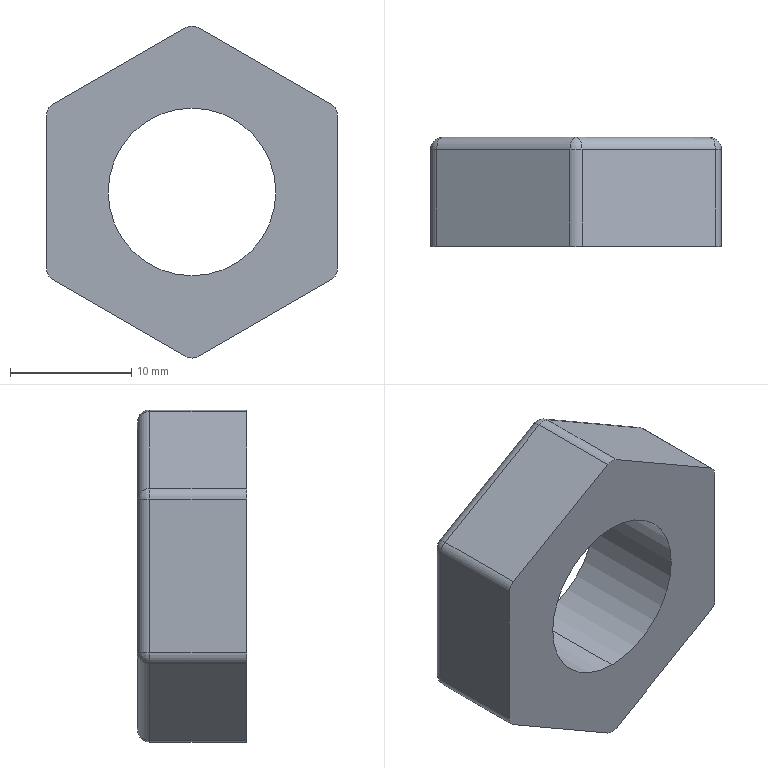Part | STEP file | NAT_Foot_GFTR16-100-100 | 1 solid | 29 faces | box 24 x 9 x 27.403 mm | volume 3116 mm3 | cylinder 15 | plane 8 | sphere 6 | commonest cylinder face diameters 2 x13 13.835 x2